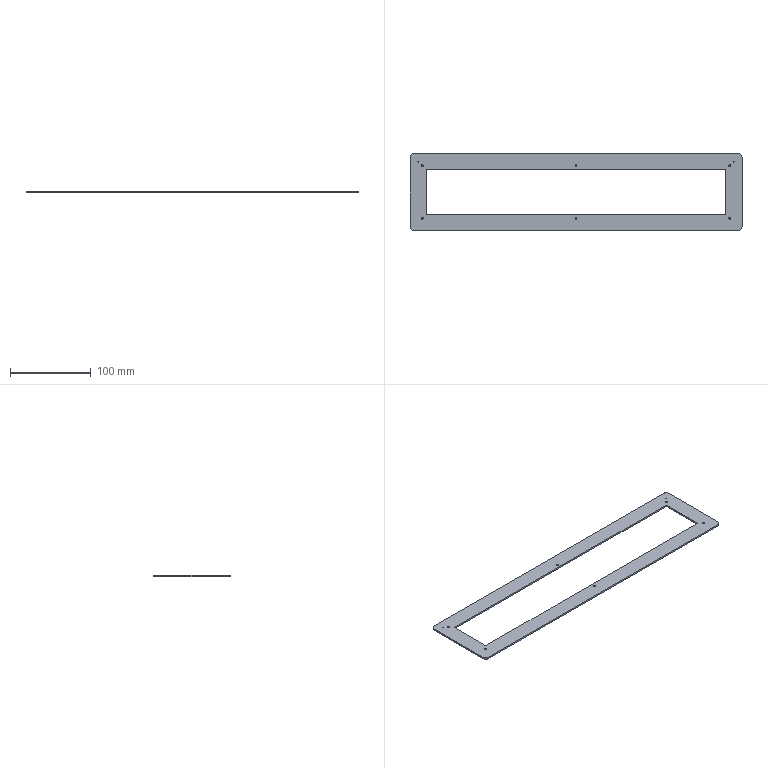Part | NX | features solid 2 | 1 solid | 30 faces | box 410 x 95 x 2 mm | volume 37097 mm3 | cylinder 20 | plane 10 | commonest cylinder face diameters 2.459 x12 1 x4 10 x4
STEP:
#1=CARTESIAN_POINT('',(-455.,-1595.5,1023.));
#2=VERTEX_POINT('',#1);
#3=CARTESIAN_POINT('',(-455.,-1595.5,1021.));
#4=VERTEX_POINT('',#3);
#5=CARTESIAN_POINT('',(-455.,-1595.5,602.133));
#6=DIRECTION('',(0.,0.,1.));
#7=VECTOR('',#6,1000.);
#8=LINE('',#5,#7);
#9=EDGE_CURVE('',#2,#4,#8,.F.);
#10=ORIENTED_EDGE('',*,*,#9,.T.);
#11=CARTESIAN_POINT('',(-455.,-1594.5,1021.));
#12=VERTEX_POINT('',#11);
#13=CARTESIAN_POINT('',(-455.,-1595.,1021.));
#14=DIRECTION('',(0.,0.,-1.));
#15=DIRECTION('',(0.,-1.,0.));
#16=AXIS2_PLACEMENT_3D('',#13,#14,#15);
#17=CIRCLE('',#16,0.5);
#18=EDGE_CURVE('',#4,#12,#17,.T.);
#19=ORIENTED_EDGE('',*,*,#18,.T.);
#20=CARTESIAN_POINT('',(-455.,-1594.5,1023.));
#21=VERTEX_POINT('',#20);
#22=CARTESIAN_POINT('',(-455.,-1594.5,602.133));
#23=DIRECTION('',(0.,0.,1.));
#24=VECTOR('',#23,1000.);
#25=LINE('',#22,#24);
#26=EDGE_CURVE('',#12,#21,#25,.T.);
#27=ORIENTED_EDGE('',*,*,#26,.T.);
#28=CARTESIAN_POINT('',(-455.,-1595.,1023.));
#29=DIRECTION('',(0.,0.,1.));
#30=DIRECTION('',(-1.,0.,0.));
#31=AXIS2_PLACEMENT_3D('',#28,#29,#30);
#32=CIRCLE('',#31,0.5);
#33=EDGE_CURVE('',#21,#2,#32,.T.);
#34=ORIENTED_EDGE('',*,*,#33,.T.);
#35=EDGE_LOOP('',(#10,#19,#27,#34));
#36=FACE_BOUND('',#35,.T.);
#37=CARTESIAN_POINT('',(-455.,-1595.,602.133));
#38=DIRECTION('',(0.,0.,1.));
#39=DIRECTION('',(0.,1.,0.));
#40=AXIS2_PLACEMENT_3D('',#37,#38,#39);
#41=CYLINDRICAL_SURFACE('',#40,0.5);
#42=ADVANCED_FACE('',(#36),#41,.F.);
#43=CARTESIAN_POINT('',(-845.,-1595.5,1023.));
#44=VERTEX_POINT('',#43);
#45=CARTESIAN_POINT('',(-845.,-1595.5,1021.));
#46=VERTEX_POINT('',#45);
#47=CARTESIAN_POINT('',(-845.,-1595.5,602.133));
#48=DIRECTION('',(0.,0.,1.));
#49=VECTOR('',#48,1000.);
#50=LINE('',#47,#49);
#51=EDGE_CURVE('',#44,#46,#50,.F.);
#52=ORIENTED_EDGE('',*,*,#51,.T.);
#53=CARTESIAN_POINT('',(-845.,-1594.5,1021.));
#54=VERTEX_POINT('',#53);
#55=CARTESIAN_POINT('',(-845.,-1595.,1021.));
#56=DIRECTION('',(0.,0.,-1.));
#57=DIRECTION('',(0.,-1.,0.));
#58=AXIS2_PLACEMENT_3D('',#55,#56,#57);
#59=CIRCLE('',#58,0.5);
#60=EDGE_CURVE('',#46,#54,#59,.T.);
#61=ORIENTED_EDGE('',*,*,#60,.T.);
#62=CARTESIAN_POINT('',(-845.,-1594.5,1023.));
#63=VERTEX_POINT('',#62);
#64=CARTESIAN_POINT('',(-845.,-1594.5,602.133));
#65=DIRECTION('',(0.,0.,1.));
#66=VECTOR('',#65,1000.);
#67=LINE('',#64,#66);
#68=EDGE_CURVE('',#54,#63,#67,.T.);
#69=ORIENTED_EDGE('',*,*,#68,.T.);
#70=CARTESIAN_POINT('',(-845.,-1595.,1023.));
#71=DIRECTION('',(0.,0.,1.));
#72=DIRECTION('',(-1.,0.,0.));
#73=AXIS2_PLACEMENT_3D('',#70,#71,#72);
#74=CIRCLE('',#73,0.5);
#75=EDGE_CURVE('',#63,#44,#74,.T.);
#76=ORIENTED_EDGE('',*,*,#75,.T.);
#77=EDGE_LOOP('',(#52,#61,#69,#76));
#78=FACE_BOUND('',#77,.T.);
#79=CARTESIAN_POINT('',(-845.,-1595.,602.133));
#80=DIRECTION('',(0.,0.,1.));
#81=DIRECTION('',(0.,1.,0.));
#82=AXIS2_PLACEMENT_3D('',#79,#80,#81);
#83=CYLINDRICAL_SURFACE('',#82,0.5);
#84=ADVANCED_FACE('',(#78),#83,.F.);
#85=CARTESIAN_POINT('',(-460.,-1598.771,1023.));
#86=VERTEX_POINT('',#85);
#87=CARTESIAN_POINT('',(-460.,-1598.771,1021.));
#88=VERTEX_POINT('',#87);
#89=CARTESIAN_POINT('',(-460.,-1598.771,1441.867));
#90=DIRECTION('',(0.,0.,-1.));
#91=VECTOR('',#90,1000.);
#92=LINE('',#89,#91);
#93=EDGE_CURVE('',#86,#88,#92,.T.);
#94=ORIENTED_EDGE('',*,*,#93,.F.);
#95=CARTESIAN_POINT('',(-460.,-1601.229,1023.));
#96=VERTEX_POINT('',#95);
#97=CARTESIAN_POINT('',(-460.,-1600.,1023.));
#98=DIRECTION('',(0.,0.,-1.));
#99=DIRECTION('',(0.,-1.,0.));
#100=AXIS2_PLACEMENT_3D('',#97,#98,#99);
#101=CIRCLE('',#100,1.23);
#102=EDGE_CURVE('',#96,#86,#101,.T.);
#103=ORIENTED_EDGE('',*,*,#102,.F.);
#104=CARTESIAN_POINT('',(-460.,-1601.229,1021.));
#105=VERTEX_POINT('',#104);
#106=CARTESIAN_POINT('',(-460.,-1601.229,1441.867));
#107=DIRECTION('',(0.,0.,-1.));
#108=VECTOR('',#107,1000.);
#109=LINE('',#106,#108);
#110=EDGE_CURVE('',#105,#96,#109,.F.);
#111=ORIENTED_EDGE('',*,*,#110,.F.);
#112=CARTESIAN_POINT('',(-460.,-1600.,1021.));
#113=DIRECTION('',(0.,0.,-1.));
#114=DIRECTION('',(-1.,0.,0.));
#115=AXIS2_PLACEMENT_3D('',#112,#113,#114);
#116=CIRCLE('',#115,1.23);
#117=EDGE_CURVE('',#105,#88,#116,.T.);
#118=ORIENTED_EDGE('',*,*,#117,.T.);
#119=EDGE_LOOP('',(#94,#103,#111,#118));
#120=FACE_BOUND('',#119,.T.);
#121=CARTESIAN_POINT('',(-460.,-1600.,1441.867));
#122=DIRECTION('',(0.,0.,-1.));
#123=DIRECTION('',(0.,-1.,0.));
#124=AXIS2_PLACEMENT_3D('',#121,#122,#123);
#125=CYLINDRICAL_SURFACE('',#124,1.23);
#126=ADVANCED_FACE('',(#120),#125,.F.);
#127=CARTESIAN_POINT('',(-460.,-1663.771,1023.));
#128=VERTEX_POINT('',#127);
#129=CARTESIAN_POINT('',(-460.,-1663.771,1021.));
#130=VERTEX_POINT('',#129);
#131=CARTESIAN_POINT('',(-460.,-1663.771,1441.867));
#132=DIRECTION('',(0.,0.,-1.));
#133=VECTOR('',#132,1000.);
#134=LINE('',#131,#133);
#135=EDGE_CURVE('',#128,#130,#134,.T.);
#136=ORIENTED_EDGE('',*,*,#135,.F.);
#137=CARTESIAN_POINT('',(-460.,-1666.229,1023.));
#138=VERTEX_POINT('',#137);
#139=CARTESIAN_POINT('',(-460.,-1665.,1023.));
#140=DIRECTION('',(0.,0.,-1.));
#141=DIRECTION('',(0.,-1.,0.));
#142=AXIS2_PLACEMENT_3D('',#139,#140,#141);
#143=CIRCLE('',#142,1.23);
#144=EDGE_CURVE('',#138,#128,#143,.T.);
#145=ORIENTED_EDGE('',*,*,#144,.F.);
#146=CARTESIAN_POINT('',(-460.,-1666.229,1021.));
#147=VERTEX_POINT('',#146);
#148=CARTESIAN_POINT('',(-460.,-1666.229,1441.867));
#149=DIRECTION('',(0.,0.,-1.));
#150=VECTOR('',#149,1000.);
#151=LINE('',#148,#150);
#152=EDGE_CURVE('',#147,#138,#151,.F.);
#153=ORIENTED_EDGE('',*,*,#152,.F.);
#154=CARTESIAN_POINT('',(-460.,-1665.,1021.));
#155=DIRECTION('',(0.,0.,-1.));
#156=DIRECTION('',(-1.,0.,0.));
#157=AXIS2_PLACEMENT_3D('',#154,#155,#156);
#158=CIRCLE('',#157,1.23);
#159=EDGE_CURVE('',#147,#130,#158,.T.);
#160=ORIENTED_EDGE('',*,*,#159,.T.);
#161=EDGE_LOOP('',(#136,#145,#153,#160));
#162=FACE_BOUND('',#161,.T.);
#163=CARTESIAN_POINT('',(-460.,-1665.,1441.867));
#164=DIRECTION('',(0.,0.,-1.));
#165=DIRECTION('',(0.,-1.,0.));
#166=AXIS2_PLACEMENT_3D('',#163,#164,#165);
#167=CYLINDRICAL_SURFACE('',#166,1.23);
#168=ADVANCED_FACE('',(#162),#167,.F.);
#169=CARTESIAN_POINT('',(-650.,-1663.771,1021.));
#170=VERTEX_POINT('',#169);
#171=CARTESIAN_POINT('',(-650.,-1663.771,1023.));
#172=VERTEX_POINT('',#171);
#173=CARTESIAN_POINT('',(-650.,-1663.771,1441.867));
#174=DIRECTION('',(0.,0.,-1.));
#175=VECTOR('',#174,1000.);
#176=LINE('',#173,#175);
#177=EDGE_CURVE('',#170,#172,#176,.F.);
#178=ORIENTED_EDGE('',*,*,#177,.T.);
#179=CARTESIAN_POINT('',(-650.,-1666.229,1023.));
#180=VERTEX_POINT('',#179);
#181=CARTESIAN_POINT('',(-650.,-1665.,1023.));
#182=DIRECTION('',(0.,0.,-1.));
#183=DIRECTION('',(0.,-1.,0.));
#184=AXIS2_PLACEMENT_3D('',#181,#182,#183);
#185=CIRCLE('',#184,1.23);
#186=EDGE_CURVE('',#180,#172,#185,.T.);
#187=ORIENTED_EDGE('',*,*,#186,.F.);
#188=CARTESIAN_POINT('',(-650.,-1666.229,1021.));
#189=VERTEX_POINT('',#188);
#190=CARTESIAN_POINT('',(-650.,-1666.229,1441.867));
#191=DIRECTION('',(0.,0.,-1.));
#192=VECTOR('',#191,1000.);
#193=LINE('',#190,#192);
#194=EDGE_CURVE('',#180,#189,#193,.T.);
#195=ORIENTED_EDGE('',*,*,#194,.T.);
#196=CARTESIAN_POINT('',(-650.,-1665.,1021.));
#197=DIRECTION('',(0.,0.,-1.));
#198=DIRECTION('',(-1.,0.,0.));
#199=AXIS2_PLACEMENT_3D('',#196,#197,#198);
#200=CIRCLE('',#199,1.23);
#201=EDGE_CURVE('',#189,#170,#200,.T.);
#202=ORIENTED_EDGE('',*,*,#201,.T.);
#203=EDGE_LOOP('',(#178,#187,#195,#202));
#204=FACE_BOUND('',#203,.T.);
#205=CARTESIAN_POINT('',(-650.,-1665.,1441.867));
#206=DIRECTION('',(0.,0.,-1.));
#207=DIRECTION('',(0.,-1.,0.));
#208=AXIS2_PLACEMENT_3D('',#205,#206,#207);
#209=CYLINDRICAL_SURFACE('',#208,1.23);
#210=ADVANCED_FACE('',(#204),#209,.F.);
#211=CARTESIAN_POINT('',(-840.,-1663.771,1021.));
#212=VERTEX_POINT('',#211);
#213=CARTESIAN_POINT('',(-840.,-1663.771,1023.));
#214=VERTEX_POINT('',#213);
#215=CARTESIAN_POINT('',(-840.,-1663.771,1441.867));
#216=DIRECTION('',(0.,0.,-1.));
#217=VECTOR('',#216,1000.);
#218=LINE('',#215,#217);
#219=EDGE_CURVE('',#212,#214,#218,.F.);
#220=ORIENTED_EDGE('',*,*,#219,.T.);
#221=CARTESIAN_POINT('',(-840.,-1666.229,1023.));
#222=VERTEX_POINT('',#221);
#223=CARTESIAN_POINT('',(-840.,-1665.,1023.));
#224=DIRECTION('',(0.,0.,-1.));
#225=DIRECTION('',(0.,-1.,0.));
#226=AXIS2_PLACEMENT_3D('',#223,#224,#225);
#227=CIRCLE('',#226,1.23);
#228=EDGE_CURVE('',#222,#214,#227,.T.);
#229=ORIENTED_EDGE('',*,*,#228,.F.);
#230=CARTESIAN_POINT('',(-840.,-1666.229,1021.));
#231=VERTEX_POINT('',#230);
#232=CARTESIAN_POINT('',(-840.,-1666.229,1441.867));
#233=DIRECTION('',(0.,0.,-1.));
#234=VECTOR('',#233,1000.);
#235=LINE('',#232,#234);
#236=EDGE_CURVE('',#222,#231,#235,.T.);
#237=ORIENTED_EDGE('',*,*,#236,.T.);
#238=CARTESIAN_POINT('',(-840.,-1665.,1021.));
#239=DIRECTION('',(0.,0.,-1.));
#240=DIRECTION('',(-1.,0.,0.));
#241=AXIS2_PLACEMENT_3D('',#238,#239,#240);
#242=CIRCLE('',#241,1.23);
#243=EDGE_CURVE('',#231,#212,#242,.T.);
#244=ORIENTED_EDGE('',*,*,#243,.T.);
#245=EDGE_LOOP('',(#220,#229,#237,#244));
#246=FACE_BOUND('',#245,.T.);
#247=CARTESIAN_POINT('',(-840.,-1665.,1441.867));
#248=DIRECTION('',(0.,0.,-1.));
#249=DIRECTION('',(0.,-1.,0.));
#250=AXIS2_PLACEMENT_3D('',#247,#248,#249);
#251=CYLINDRICAL_SURFACE('',#250,1.23);
#252=ADVANCED_FACE('',(#246),#251,.F.);
#253=CARTESIAN_POINT('',(-840.,-1598.771,1021.));
#254=VERTEX_POINT('',#253);
#255=CARTESIAN_POINT('',(-840.,-1598.771,1023.));
#256=VERTEX_POINT('',#255);
#257=CARTESIAN_POINT('',(-840.,-1598.771,1441.867));
#258=DIRECTION('',(0.,0.,-1.));
#259=VECTOR('',#258,1000.);
#260=LINE('',#257,#259);
#261=EDGE_CURVE('',#254,#256,#260,.F.);
#262=ORIENTED_EDGE('',*,*,#261,.T.);
#263=CARTESIAN_POINT('',(-840.,-1601.229,1023.));
#264=VERTEX_POINT('',#263);
#265=CARTESIAN_POINT('',(-840.,-1600.,1023.));
#266=DIRECTION('',(0.,0.,-1.));
#267=DIRECTION('',(0.,-1.,0.));
#268=AXIS2_PLACEMENT_3D('',#265,#266,#267);
#269=CIRCLE('',#268,1.23);
#270=EDGE_CURVE('',#264,#256,#269,.T.);
#271=ORIENTED_EDGE('',*,*,#270,.F.);
#272=CARTESIAN_POINT('',(-840.,-1601.229,1021.));
#273=VERTEX_POINT('',#272);
#274=CARTESIAN_POINT('',(-840.,-1601.229,1441.867));
#275=DIRECTION('',(0.,0.,-1.));
#276=VECTOR('',#275,1000.);
#277=LINE('',#274,#276);
#278=EDGE_CURVE('',#264,#273,#277,.T.);
#279=ORIENTED_EDGE('',*,*,#278,.T.);
#280=CARTESIAN_POINT('',(-840.,-1600.,1021.));
#281=DIRECTION('',(0.,0.,-1.));
#282=DIRECTION('',(-1.,0.,0.));
#283=AXIS2_PLACEMENT_3D('',#280,#281,#282);
#284=CIRCLE('',#283,1.23);
#285=EDGE_CURVE('',#273,#254,#284,.T.);
#286=ORIENTED_EDGE('',*,*,#285,.T.);
#287=EDGE_LOOP('',(#262,#271,#279,#286));
#288=FACE_BOUND('',#287,.T.);
#289=CARTESIAN_POINT('',(-840.,-1600.,1441.867));
#290=DIRECTION('',(0.,0.,-1.));
#291=DIRECTION('',(0.,-1.,0.));
#292=AXIS2_PLACEMENT_3D('',#289,#290,#291);
#293=CYLINDRICAL_SURFACE('',#292,1.23);
#294=ADVANCED_FACE('',(#288),#293,.F.);
#295=CARTESIAN_POINT('',(-650.,-1598.771,1021.));
#296=VERTEX_POINT('',#295);
#297=CARTESIAN_POINT('',(-650.,-1598.771,1023.));
#298=VERTEX_POINT('',#297);
#299=CARTESIAN_POINT('',(-650.,-1598.771,1441.867));
#300=DIRECTION('',(0.,0.,-1.));
#301=VECTOR('',#300,1000.);
#302=LINE('',#299,#301);
#303=EDGE_CURVE('',#296,#298,#302,.F.);
#304=ORIENTED_EDGE('',*,*,#303,.T.);
#305=CARTESIAN_POINT('',(-650.,-1601.229,1023.));
#306=VERTEX_POINT('',#305);
#307=CARTESIAN_POINT('',(-650.,-1600.,1023.));
#308=DIRECTION('',(0.,0.,-1.));
#309=DIRECTION('',(0.,-1.,0.));
#310=AXIS2_PLACEMENT_3D('',#307,#308,#309);
#311=CIRCLE('',#310,1.23);
#312=EDGE_CURVE('',#306,#298,#311,.T.);
#313=ORIENTED_EDGE('',*,*,#312,.F.);
#314=CARTESIAN_POINT('',(-650.,-1601.229,1021.));
#315=VERTEX_POINT('',#314);
#316=CARTESIAN_POINT('',(-650.,-1601.229,1441.867));
#317=DIRECTION('',(0.,0.,-1.));
#318=VECTOR('',#317,1000.);
#319=LINE('',#316,#318);
#320=EDGE_CURVE('',#306,#315,#319,.T.);
#321=ORIENTED_EDGE('',*,*,#320,.T.);
#322=CARTESIAN_POINT('',(-650.,-1600.,1021.));
#323=DIRECTION('',(0.,0.,-1.));
#324=DIRECTION('',(-1.,0.,0.));
#325=AXIS2_PLACEMENT_3D('',#322,#323,#324);
#326=CIRCLE('',#325,1.23);
#327=EDGE_CURVE('',#315,#296,#326,.T.);
#328=ORIENTED_EDGE('',*,*,#327,.T.);
#329=EDGE_LOOP('',(#304,#313,#321,#328));
#330=FACE_BOUND('',#329,.T.);
#331=CARTESIAN_POINT('',(-650.,-1600.,1441.867));
#332=DIRECTION('',(0.,0.,-1.));
#333=DIRECTION('',(0.,-1.,0.));
#334=AXIS2_PLACEMENT_3D('',#331,#332,#333);
#335=CYLINDRICAL_SURFACE('',#334,1.23);
#336=ADVANCED_FACE('',(#330),#335,.F.);
#337=CARTESIAN_POINT('',(-850.,-1585.,1023.));
#338=VERTEX_POINT('',#337);
#339=CARTESIAN_POINT('',(-855.,-1590.,1023.));
#340=VERTEX_POINT('',#339);
#341=CARTESIAN_POINT('',(-850.,-1590.,1023.));
#342=DIRECTION('',(0.,0.,1.));
#343=DIRECTION('',(0.,-1.,0.));
#344=AXIS2_PLACEMENT_3D('',#341,#342,#343);
#345=CIRCLE('',#344,5.);
#346=EDGE_CURVE('',#338,#340,#345,.T.);
#347=ORIENTED_EDGE('',*,*,#346,.F.);
#348=CARTESIAN_POINT('',(-850.,-1585.,1021.));
#349=VERTEX_POINT('',#348);
#350=CARTESIAN_POINT('',(-850.,-1585.,1023.));
#351=DIRECTION('',(0.,0.,1.));
#352=VECTOR('',#351,1000.);
#353=LINE('',#350,#352);
#354=EDGE_CURVE('',#349,#338,#353,.T.);
#355=ORIENTED_EDGE('',*,*,#354,.F.);
#356=CARTESIAN_POINT('',(-855.,-1590.,1021.));
#357=VERTEX_POINT('',#356);
#358=CARTESIAN_POINT('',(-850.,-1590.,1021.));
#359=DIRECTION('',(0.,0.,-1.));
#360=DIRECTION('',(0.,-1.,0.));
#361=AXIS2_PLACEMENT_3D('',#358,#359,#360);
#362=CIRCLE('',#361,5.);
#363=EDGE_CURVE('',#357,#349,#362,.T.);
#364=ORIENTED_EDGE('',*,*,#363,.F.);
#365=CARTESIAN_POINT('',(-855.,-1590.,1023.));
#366=DIRECTION('',(0.,0.,-1.));
#367=VECTOR('',#366,1000.);
#368=LINE('',#365,#367);
#369=EDGE_CURVE('',#340,#357,#368,.T.);
#370=ORIENTED_EDGE('',*,*,#369,.F.);
#371=EDGE_LOOP('',(#347,#355,#364,#370));
#372=FACE_BOUND('',#371,.T.);
#373=CARTESIAN_POINT('',(-850.,-1590.,1023.));
#374=DIRECTION('',(0.,0.,-1.));
#375=DIRECTION('',(0.,-1.,0.));
#376=AXIS2_PLACEMENT_3D('',#373,#374,#375);
#377=CYLINDRICAL_SURFACE('',#376,5.);
#378=ADVANCED_FACE('',(#372),#377,.T.);
#379=CARTESIAN_POINT('',(-450.,-1680.,1023.));
#380=VERTEX_POINT('',#379);
#381=CARTESIAN_POINT('',(-445.,-1675.,1023.));
#382=VERTEX_POINT('',#381);
#383=CARTESIAN_POINT('',(-450.,-1675.,1023.));
#384=DIRECTION('',(0.,0.,1.));
#385=DIRECTION('',(0.,-1.,0.));
#386=AXIS2_PLACEMENT_3D('',#383,#384,#385);
#387=CIRCLE('',#386,5.);
#388=EDGE_CURVE('',#380,#382,#387,.T.);
#389=ORIENTED_EDGE('',*,*,#388,.F.);
#390=CARTESIAN_POINT('',(-450.,-1680.,1021.));
#391=VERTEX_POINT('',#390);
#392=CARTESIAN_POINT('',(-450.,-1680.,1023.));
#393=DIRECTION('',(0.,0.,1.));
#394=VECTOR('',#393,1000.);
#395=LINE('',#392,#394);
#396=EDGE_CURVE('',#391,#380,#395,.T.);
#397=ORIENTED_EDGE('',*,*,#396,.F.);
#398=CARTESIAN_POINT('',(-445.,-1675.,1021.));
#399=VERTEX_POINT('',#398);
#400=CARTESIAN_POINT('',(-450.,-1675.,1021.));
#401=DIRECTION('',(0.,0.,-1.));
#402=DIRECTION('',(0.,-1.,0.));
#403=AXIS2_PLACEMENT_3D('',#400,#401,#402);
#404=CIRCLE('',#403,5.);
#405=EDGE_CURVE('',#399,#391,#404,.T.);
#406=ORIENTED_EDGE('',*,*,#405,.F.);
#407=CARTESIAN_POINT('',(-445.,-1675.,1023.));
#408=DIRECTION('',(0.,0.,-1.));
#409=VECTOR('',#408,1000.);
#410=LINE('',#407,#409);
#411=EDGE_CURVE('',#382,#399,#410,.T.);
#412=ORIENTED_EDGE('',*,*,#411,.F.);
#413=EDGE_LOOP('',(#389,#397,#406,#412));
#414=FACE_BOUND('',#413,.T.);
#415=CARTESIAN_POINT('',(-450.,-1675.,1023.));
#416=DIRECTION('',(0.,0.,-1.));
#417=DIRECTION('',(0.,-1.,0.));
#418=AXIS2_PLACEMENT_3D('',#415,#416,#417);
#419=CYLINDRICAL_SURFACE('',#418,5.);
#420=ADVANCED_FACE('',(#414),#419,.T.);
#421=CARTESIAN_POINT('',(-445.,-1590.,1023.));
#422=VERTEX_POINT('',#421);
#423=CARTESIAN_POINT('',(-450.,-1585.,1023.));
#424=VERTEX_POINT('',#423);
#425=CARTESIAN_POINT('',(-450.,-1590.,1023.));
#426=DIRECTION('',(0.,0.,1.));
#427=DIRECTION('',(0.,-1.,0.));
#428=AXIS2_PLACEMENT_3D('',#425,#426,#427);
#429=CIRCLE('',#428,5.);
#430=EDGE_CURVE('',#422,#424,#429,.T.);
#431=ORIENTED_EDGE('',*,*,#430,.F.);
#432=CARTESIAN_POINT('',(-445.,-1590.,1021.));
#433=VERTEX_POINT('',#432);
#434=CARTESIAN_POINT('',(-445.,-1590.,1023.));
#435=DIRECTION('',(0.,0.,1.));
#436=VECTOR('',#435,1000.);
#437=LINE('',#434,#436);
#438=EDGE_CURVE('',#433,#422,#437,.T.);
#439=ORIENTED_EDGE('',*,*,#438,.F.);
#440=CARTESIAN_POINT('',(-450.,-1585.,1021.));
#441=VERTEX_POINT('',#440);
#442=CARTESIAN_POINT('',(-450.,-1590.,1021.));
#443=DIRECTION('',(0.,0.,-1.));
#444=DIRECTION('',(0.,-1.,0.));
#445=AXIS2_PLACEMENT_3D('',#442,#443,#444);
#446=CIRCLE('',#445,5.);
#447=EDGE_CURVE('',#441,#433,#446,.T.);
#448=ORIENTED_EDGE('',*,*,#447,.F.);
#449=CARTESIAN_POINT('',(-450.,-1585.,1023.));
#450=DIRECTION('',(0.,0.,-1.));
#451=VECTOR('',#450,1000.);
#452=LINE('',#449,#451);
#453=EDGE_CURVE('',#424,#441,#452,.T.);
#454=ORIENTED_EDGE('',*,*,#453,.F.);
#455=EDGE_LOOP('',(#431,#439,#448,#454));
#456=FACE_BOUND('',#455,.T.);
#457=CARTESIAN_POINT('',(-450.,-1590.,1023.));
#458=DIRECTION('',(0.,0.,-1.));
#459=DIRECTION('',(0.,-1.,0.));
#460=AXIS2_PLACEMENT_3D('',#457,#458,#459);
#461=CYLINDRICAL_SURFACE('',#460,5.);
#462=ADVANCED_FACE('',(#456),#461,.T.);
#463=CARTESIAN_POINT('',(-855.,-1675.,1023.));
#464=VERTEX_POINT('',#463);
#465=CARTESIAN_POINT('',(-850.,-1680.,1023.));
#466=VERTEX_POINT('',#465);
#467=CARTESIAN_POINT('',(-850.,-1675.,1023.));
#468=DIRECTION('',(0.,0.,1.));
#469=DIRECTION('',(0.,-1.,0.));
#470=AXIS2_PLACEMENT_3D('',#467,#468,#469);
#471=CIRCLE('',#470,5.);
#472=EDGE_CURVE('',#464,#466,#471,.T.);
#473=ORIENTED_EDGE('',*,*,#472,.F.);
#474=CARTESIAN_POINT('',(-855.,-1675.,1021.));
#475=VERTEX_POINT('',#474);
#476=CARTESIAN_POINT('',(-855.,-1675.,1023.));
#477=DIRECTION('',(0.,0.,1.));
#478=VECTOR('',#477,1000.);
#479=LINE('',#476,#478);
#480=EDGE_CURVE('',#475,#464,#479,.T.);
#481=ORIENTED_EDGE('',*,*,#480,.F.);
#482=CARTESIAN_POINT('',(-850.,-1680.,1021.));
#483=VERTEX_POINT('',#482);
#484=CARTESIAN_POINT('',(-850.,-1675.,1021.));
#485=DIRECTION('',(0.,0.,-1.));
#486=DIRECTION('',(0.,-1.,0.));
#487=AXIS2_PLACEMENT_3D('',#484,#485,#486);
#488=CIRCLE('',#487,5.);
#489=EDGE_CURVE('',#483,#475,#488,.T.);
#490=ORIENTED_EDGE('',*,*,#489,.F.);
#491=CARTESIAN_POINT('',(-850.,-1680.,1023.));
#492=DIRECTION('',(0.,0.,-1.));
#493=VECTOR('',#492,1000.);
#494=LINE('',#491,#493);
#495=EDGE_CURVE('',#466,#483,#494,.T.);
#496=ORIENTED_EDGE('',*,*,#495,.F.);
#497=EDGE_LOOP('',(#473,#481,#490,#496));
#498=FACE_BOUND('',#497,.T.);
#499=CARTESIAN_POINT('',(-850.,-1675.,1023.));
#500=DIRECTION('',(0.,0.,-1.));
#501=DIRECTION('',(0.,-1.,0.));
#502=AXIS2_PLACEMENT_3D('',#499,#500,#501);
#503=CYLINDRICAL_SURFACE('',#502,5.);
#504=ADVANCED_FACE('',(#498),#503,.T.);
#505=CARTESIAN_POINT('',(-835.,-1605.,1023.));
#506=VERTEX_POINT('',#505);
#507=CARTESIAN_POINT('',(-835.,-1605.,1021.));
#508=VERTEX_POINT('',#507);
#509=CARTESIAN_POINT('',(-835.,-1605.,1441.867));
#510=DIRECTION('',(0.,0.,-1.));
#511=VECTOR('',#510,1000.);
#512=LINE('',#509,#511);
#513=EDGE_CURVE('',#506,#508,#512,.T.);
#514=ORIENTED_EDGE('',*,*,#513,.T.);
#515=CARTESIAN_POINT('',(-465.,-1605.,1021.));
#516=VERTEX_POINT('',#515);
#517=CARTESIAN_POINT('',(-835.,-1605.,1021.));
#518=DIRECTION('',(1.,0.,0.));
#519=VECTOR('',#518,1000.);
#520=LINE('',#517,#519);
#521=EDGE_CURVE('',#508,#516,#520,.T.);
#522=ORIENTED_EDGE('',*,*,#521,.T.);
#523=CARTESIAN_POINT('',(-465.,-1605.,1023.));
#524=VERTEX_POINT('',#523);
#525=CARTESIAN_POINT('',(-465.,-1605.,1441.867));
#526=DIRECTION('',(0.,0.,-1.));
#527=VECTOR('',#526,1000.);
#528=LINE('',#525,#527);
#529=EDGE_CURVE('',#524,#516,#528,.T.);
#530=ORIENTED_EDGE('',*,*,#529,.F.);
#531=CARTESIAN_POINT('',(-445.,-1605.,1023.));
#532=DIRECTION('',(1.,0.,0.));
#533=VECTOR('',#532,1000.);
#534=LINE('',#531,#533);
#535=EDGE_CURVE('',#506,#524,#534,.T.);
#536=ORIENTED_EDGE('',*,*,#535,.F.);
#537=EDGE_LOOP('',(#514,#522,#530,#536));
#538=FACE_BOUND('',#537,.T.);
#539=CARTESIAN_POINT('',(-835.,-1605.,1441.867));
#540=DIRECTION('',(0.,1.,0.));
#541=DIRECTION('',(0.,0.,-1.));
#542=AXIS2_PLACEMENT_3D('',#539,#540,#541);
#543=PLANE('',#542);
#544=ADVANCED_FACE('',(#538),#543,.F.);
#545=CARTESIAN_POINT('',(-835.,-1660.,1023.));
#546=VERTEX_POINT('',#545);
#547=CARTESIAN_POINT('',(-835.,-1660.,1021.));
#548=VERTEX_POINT('',#547);
#549=CARTESIAN_POINT('',(-835.,-1660.,1441.867));
#550=DIRECTION('',(0.,0.,-1.));
#551=VECTOR('',#550,1000.);
#552=LINE('',#549,#551);
#553=EDGE_CURVE('',#546,#548,#552,.T.);
#554=ORIENTED_EDGE('',*,*,#553,.T.);
#555=CARTESIAN_POINT('',(-835.,-1660.,1021.));
#556=DIRECTION('',(0.,1.,0.));
#557=VECTOR('',#556,1000.);
#558=LINE('',#555,#557);
#559=EDGE_CURVE('',#548,#508,#558,.T.);
#560=ORIENTED_EDGE('',*,*,#559,.T.);
#561=ORIENTED_EDGE('',*,*,#513,.F.);
#562=CARTESIAN_POINT('',(-835.,-1680.,1023.));
#563=DIRECTION('',(0.,1.,0.));
#564=VECTOR('',#563,1000.);
#565=LINE('',#562,#564);
#566=EDGE_CURVE('',#546,#506,#565,.T.);
#567=ORIENTED_EDGE('',*,*,#566,.F.);
#568=EDGE_LOOP('',(#554,#560,#561,#567));
#569=FACE_BOUND('',#568,.T.);
#570=CARTESIAN_POINT('',(-835.,-1660.,1441.867));
#571=DIRECTION('',(-1.,0.,0.));
#572=DIRECTION('',(0.,1.,0.));
#573=AXIS2_PLACEMENT_3D('',#570,#571,#572);
#574=PLANE('',#573);
#575=ADVANCED_FACE('',(#569),#574,.F.);
#576=CARTESIAN_POINT('',(-465.,-1660.,1023.));
#577=VERTEX_POINT('',#576);
#578=CARTESIAN_POINT('',(-465.,-1660.,1021.));
#579=VERTEX_POINT('',#578);
#580=CARTESIAN_POINT('',(-465.,-1660.,1441.867));
#581=DIRECTION('',(0.,0.,-1.));
#582=VECTOR('',#581,1000.);
#583=LINE('',#580,#582);
#584=EDGE_CURVE('',#577,#579,#583,.T.);
#585=ORIENTED_EDGE('',*,*,#584,.T.);
#586=CARTESIAN_POINT('',(-465.,-1660.,1021.));
#587=DIRECTION('',(-1.,0.,0.));
#588=VECTOR('',#587,1000.);
#589=LINE('',#586,#588);
#590=EDGE_CURVE('',#579,#548,#589,.T.);
#591=ORIENTED_EDGE('',*,*,#590,.T.);
#592=ORIENTED_EDGE('',*,*,#553,.F.);
#593=CARTESIAN_POINT('',(-445.,-1660.,1023.));
#594=DIRECTION('',(-1.,0.,0.));
#595=VECTOR('',#594,1000.);
#596=LINE('',#593,#595);
#597=EDGE_CURVE('',#577,#546,#596,.T.);
#598=ORIENTED_EDGE('',*,*,#597,.F.);
#599=EDGE_LOOP('',(#585,#591,#592,#598));
#600=FACE_BOUND('',#599,.T.);
#601=CARTESIAN_POINT('',(-465.,-1660.,1441.867));
#602=DIRECTION('',(0.,-1.,0.));
#603=DIRECTION('',(-1.,0.,0.));
#604=AXIS2_PLACEMENT_3D('',#601,#602,#603);
#605=PLANE('',#604);
#606=ADVANCED_FACE('',(#600),#605,.F.);
#607=ORIENTED_EDGE('',*,*,#529,.T.);
#608=CARTESIAN_POINT('',(-465.,-1605.,1021.));
#609=DIRECTION('',(0.,-1.,0.));
#610=VECTOR('',#609,1000.);
#611=LINE('',#608,#610);
#612=EDGE_CURVE('',#516,#579,#611,.T.);
#613=ORIENTED_EDGE('',*,*,#612,.T.);
#614=ORIENTED_EDGE('',*,*,#584,.F.);
#615=CARTESIAN_POINT('',(-465.,-1680.,1023.));
#616=DIRECTION('',(0.,-1.,0.));
#617=VECTOR('',#616,1000.);
#618=LINE('',#615,#617);
#619=EDGE_CURVE('',#524,#577,#618,.T.);
#620=ORIENTED_EDGE('',*,*,#619,.F.);
#621=EDGE_LOOP('',(#607,#613,#614,#620));
#622=FACE_BOUND('',#621,.T.);
#623=CARTESIAN_POINT('',(-465.,-1605.,1441.867));
#624=DIRECTION('',(1.,0.,0.));
#625=DIRECTION('',(0.,0.,-1.));
#626=AXIS2_PLACEMENT_3D('',#623,#624,#625);
#627=PLANE('',#626);
#628=ADVANCED_FACE('',(#622),#627,.F.);
#629=ORIENTED_EDGE('',*,*,#612,.F.);
#630=ORIENTED_EDGE('',*,*,#521,.F.);
#631=ORIENTED_EDGE('',*,*,#559,.F.);
#632=ORIENTED_EDGE('',*,*,#590,.F.);
#633=EDGE_LOOP('',(#629,#630,#631,#632));
#634=FACE_BOUND('',#633,.T.);
#635=ORIENTED_EDGE('',*,*,#327,.F.);
#636=CARTESIAN_POINT('',(-650.,-1600.,1021.));
#637=DIRECTION('',(0.,0.,-1.));
#638=DIRECTION('',(-1.,0.,0.));
#639=AXIS2_PLACEMENT_3D('',#636,#637,#638);
#640=CIRCLE('',#639,1.23);
#641=EDGE_CURVE('',#296,#315,#640,.T.);
#642=ORIENTED_EDGE('',*,*,#641,.F.);
#643=EDGE_LOOP('',(#635,#642));
#644=FACE_BOUND('',#643,.T.);
#645=ORIENTED_EDGE('',*,*,#285,.F.);
#646=CARTESIAN_POINT('',(-840.,-1600.,1021.));
#647=DIRECTION('',(0.,0.,-1.));
#648=DIRECTION('',(-1.,0.,0.));
#649=AXIS2_PLACEMENT_3D('',#646,#647,#648);
#650=CIRCLE('',#649,1.23);
#651=EDGE_CURVE('',#254,#273,#650,.T.);
#652=ORIENTED_EDGE('',*,*,#651,.F.);
#653=EDGE_LOOP('',(#645,#652));
#654=FACE_BOUND('',#653,.T.);
#655=ORIENTED_EDGE('',*,*,#243,.F.);
#656=CARTESIAN_POINT('',(-840.,-1665.,1021.));
#657=DIRECTION('',(0.,0.,-1.));
#658=DIRECTION('',(-1.,0.,0.));
#659=AXIS2_PLACEMENT_3D('',#656,#657,#658);
#660=CIRCLE('',#659,1.23);
#661=EDGE_CURVE('',#212,#231,#660,.T.);
#662=ORIENTED_EDGE('',*,*,#661,.F.);
#663=EDGE_LOOP('',(#655,#662));
#664=FACE_BOUND('',#663,.T.);
#665=ORIENTED_EDGE('',*,*,#201,.F.);
#666=CARTESIAN_POINT('',(-650.,-1665.,1021.));
#667=DIRECTION('',(0.,0.,-1.));
#668=DIRECTION('',(-1.,0.,0.));
#669=AXIS2_PLACEMENT_3D('',#666,#667,#668);
#670=CIRCLE('',#669,1.23);
#671=EDGE_CURVE('',#170,#189,#670,.T.);
#672=ORIENTED_EDGE('',*,*,#671,.F.);
#673=EDGE_LOOP('',(#665,#672));
#674=FACE_BOUND('',#673,.T.);
#675=ORIENTED_EDGE('',*,*,#159,.F.);
#676=CARTESIAN_POINT('',(-460.,-1665.,1021.));
#677=DIRECTION('',(0.,0.,-1.));
#678=DIRECTION('',(-1.,0.,0.));
#679=AXIS2_PLACEMENT_3D('',#676,#677,#678);
#680=CIRCLE('',#679,1.23);
#681=EDGE_CURVE('',#130,#147,#680,.T.);
#682=ORIENTED_EDGE('',*,*,#681,.F.);
#683=EDGE_LOOP('',(#675,#682));
#684=FACE_BOUND('',#683,.T.);
#685=ORIENTED_EDGE('',*,*,#117,.F.);
#686=CARTESIAN_POINT('',(-460.,-1600.,1021.));
#687=DIRECTION('',(0.,0.,-1.));
#688=DIRECTION('',(-1.,0.,0.));
#689=AXIS2_PLACEMENT_3D('',#686,#687,#688);
#690=CIRCLE('',#689,1.23);
#691=EDGE_CURVE('',#88,#105,#690,.T.);
#692=ORIENTED_EDGE('',*,*,#691,.F.);
#693=EDGE_LOOP('',(#685,#692));
#694=FACE_BOUND('',#693,.T.);
#695=CARTESIAN_POINT('',(-845.,-1595.,1021.));
#696=DIRECTION('',(0.,0.,-1.));
#697=DIRECTION('',(0.,-1.,0.));
#698=AXIS2_PLACEMENT_3D('',#695,#696,#697);
#699=CIRCLE('',#698,0.5);
#700=EDGE_CURVE('',#54,#46,#699,.T.);
#701=ORIENTED_EDGE('',*,*,#700,.F.);
#702=ORIENTED_EDGE('',*,*,#60,.F.);
#703=EDGE_LOOP('',(#701,#702));
#704=FACE_BOUND('',#703,.T.);
#705=CARTESIAN_POINT('',(-455.,-1595.,1021.));
#706=DIRECTION('',(0.,0.,-1.));
#707=DIRECTION('',(0.,-1.,0.));
#708=AXIS2_PLACEMENT_3D('',#705,#706,#707);
#709=CIRCLE('',#708,0.5);
#710=EDGE_CURVE('',#12,#4,#709,.T.);
#711=ORIENTED_EDGE('',*,*,#710,.F.);
#712=ORIENTED_EDGE('',*,*,#18,.F.);
#713=EDGE_LOOP('',(#711,#712));
#714=FACE_BOUND('',#713,.T.);
#715=CARTESIAN_POINT('',(-445.,-1680.,1021.));
#716=DIRECTION('',(-1.,0.,0.));
#717=VECTOR('',#716,1000.);
#718=LINE('',#715,#717);
#719=EDGE_CURVE('',#391,#483,#718,.T.);
#720=ORIENTED_EDGE('',*,*,#719,.T.);
#721=ORIENTED_EDGE('',*,*,#489,.T.);
#722=CARTESIAN_POINT('',(-855.,-1680.,1021.));
#723=DIRECTION('',(0.,1.,0.));
#724=VECTOR('',#723,1000.);
#725=LINE('',#722,#724);
#726=EDGE_CURVE('',#475,#357,#725,.T.);
#727=ORIENTED_EDGE('',*,*,#726,.T.);
#728=ORIENTED_EDGE('',*,*,#363,.T.);
#729=CARTESIAN_POINT('',(-855.,-1585.,1021.));
#730=DIRECTION('',(1.,0.,0.));
#731=VECTOR('',#730,1000.);
#732=LINE('',#729,#731);
#733=EDGE_CURVE('',#349,#441,#732,.T.);
#734=ORIENTED_EDGE('',*,*,#733,.T.);
#735=ORIENTED_EDGE('',*,*,#447,.T.);
#736=CARTESIAN_POINT('',(-445.,-1585.,1021.));
#737=DIRECTION('',(0.,-1.,0.));
#738=VECTOR('',#737,1000.);
#739=LINE('',#736,#738);
#740=EDGE_CURVE('',#433,#399,#739,.T.);
#741=ORIENTED_EDGE('',*,*,#740,.T.);
#742=ORIENTED_EDGE('',*,*,#405,.T.);
#743=EDGE_LOOP('',(#720,#721,#727,#728,#734,#735,#741,#742));
#744=FACE_BOUND('',#743,.T.);
#745=CARTESIAN_POINT('',(-445.,-1680.,1021.));
#746=DIRECTION('',(0.,0.,-1.));
#747=DIRECTION('',(0.,-1.,0.));
#748=AXIS2_PLACEMENT_3D('',#745,#746,#747);
#749=PLANE('',#748);
#750=ADVANCED_FACE('',(#634,#644,#654,#664,#674,#684,#694,#704,#714,#744),#749,.T.);
#751=ORIENTED_EDGE('',*,*,#535,.T.);
#752=ORIENTED_EDGE('',*,*,#619,.T.);
#753=ORIENTED_EDGE('',*,*,#597,.T.);
#754=ORIENTED_EDGE('',*,*,#566,.T.);
#755=EDGE_LOOP('',(#751,#752,#753,#754));
#756=FACE_BOUND('',#755,.T.);
#757=ORIENTED_EDGE('',*,*,#312,.T.);
#758=CARTESIAN_POINT('',(-650.,-1600.,1023.));
#759=DIRECTION('',(0.,0.,-1.));
#760=DIRECTION('',(0.,-1.,0.));
#761=AXIS2_PLACEMENT_3D('',#758,#759,#760);
#762=CIRCLE('',#761,1.23);
#763=EDGE_CURVE('',#298,#306,#762,.T.);
#764=ORIENTED_EDGE('',*,*,#763,.T.);
#765=EDGE_LOOP('',(#757,#764));
#766=FACE_BOUND('',#765,.T.);
#767=ORIENTED_EDGE('',*,*,#270,.T.);
#768=CARTESIAN_POINT('',(-840.,-1600.,1023.));
#769=DIRECTION('',(0.,0.,-1.));
#770=DIRECTION('',(0.,-1.,0.));
#771=AXIS2_PLACEMENT_3D('',#768,#769,#770);
#772=CIRCLE('',#771,1.23);
#773=EDGE_CURVE('',#256,#264,#772,.T.);
#774=ORIENTED_EDGE('',*,*,#773,.T.);
#775=EDGE_LOOP('',(#767,#774));
#776=FACE_BOUND('',#775,.T.);
#777=ORIENTED_EDGE('',*,*,#228,.T.);
#778=CARTESIAN_POINT('',(-840.,-1665.,1023.));
#779=DIRECTION('',(0.,0.,-1.));
#780=DIRECTION('',(0.,-1.,0.));
#781=AXIS2_PLACEMENT_3D('',#778,#779,#780);
#782=CIRCLE('',#781,1.23);
#783=EDGE_CURVE('',#214,#222,#782,.T.);
#784=ORIENTED_EDGE('',*,*,#783,.T.);
#785=EDGE_LOOP('',(#777,#784));
#786=FACE_BOUND('',#785,.T.);
#787=ORIENTED_EDGE('',*,*,#186,.T.);
#788=CARTESIAN_POINT('',(-650.,-1665.,1023.));
#789=DIRECTION('',(0.,0.,-1.));
#790=DIRECTION('',(0.,-1.,0.));
#791=AXIS2_PLACEMENT_3D('',#788,#789,#790);
#792=CIRCLE('',#791,1.23);
#793=EDGE_CURVE('',#172,#180,#792,.T.);
#794=ORIENTED_EDGE('',*,*,#793,.T.);
#795=EDGE_LOOP('',(#787,#794));
#796=FACE_BOUND('',#795,.T.);
#797=ORIENTED_EDGE('',*,*,#144,.T.);
#798=CARTESIAN_POINT('',(-460.,-1665.,1023.));
#799=DIRECTION('',(0.,0.,-1.));
#800=DIRECTION('',(0.,-1.,0.));
#801=AXIS2_PLACEMENT_3D('',#798,#799,#800);
#802=CIRCLE('',#801,1.23);
#803=EDGE_CURVE('',#128,#138,#802,.T.);
#804=ORIENTED_EDGE('',*,*,#803,.T.);
#805=EDGE_LOOP('',(#797,#804));
#806=FACE_BOUND('',#805,.T.);
#807=ORIENTED_EDGE('',*,*,#102,.T.);
#808=CARTESIAN_POINT('',(-460.,-1600.,1023.));
#809=DIRECTION('',(0.,0.,-1.));
#810=DIRECTION('',(0.,-1.,0.));
#811=AXIS2_PLACEMENT_3D('',#808,#809,#810);
#812=CIRCLE('',#811,1.23);
#813=EDGE_CURVE('',#86,#96,#812,.T.);
#814=ORIENTED_EDGE('',*,*,#813,.T.);
#815=EDGE_LOOP('',(#807,#814));
#816=FACE_BOUND('',#815,.T.);
#817=ORIENTED_EDGE('',*,*,#75,.F.);
#818=CARTESIAN_POINT('',(-845.,-1595.,1023.));
#819=DIRECTION('',(0.,0.,1.));
#820=DIRECTION('',(-1.,0.,0.));
#821=AXIS2_PLACEMENT_3D('',#818,#819,#820);
#822=CIRCLE('',#821,0.5);
#823=EDGE_CURVE('',#44,#63,#822,.T.);
#824=ORIENTED_EDGE('',*,*,#823,.F.);
#825=EDGE_LOOP('',(#817,#824));
#826=FACE_BOUND('',#825,.T.);
#827=ORIENTED_EDGE('',*,*,#33,.F.);
#828=CARTESIAN_POINT('',(-455.,-1595.,1023.));
#829=DIRECTION('',(0.,0.,1.));
#830=DIRECTION('',(-1.,0.,0.));
#831=AXIS2_PLACEMENT_3D('',#828,#829,#830);
#832=CIRCLE('',#831,0.5);
#833=EDGE_CURVE('',#2,#21,#832,.T.);
#834=ORIENTED_EDGE('',*,*,#833,.F.);
#835=EDGE_LOOP('',(#827,#834));
#836=FACE_BOUND('',#835,.T.);
#837=CARTESIAN_POINT('',(-855.,-1680.,1023.));
#838=DIRECTION('',(0.,1.,0.));
#839=VECTOR('',#838,1000.);
#840=LINE('',#837,#839);
#841=EDGE_CURVE('',#464,#340,#840,.T.);
#842=ORIENTED_EDGE('',*,*,#841,.F.);
#843=ORIENTED_EDGE('',*,*,#472,.T.);
#844=CARTESIAN_POINT('',(-445.,-1680.,1023.));
#845=DIRECTION('',(-1.,0.,0.));
#846=VECTOR('',#845,1000.);
#847=LINE('',#844,#846);
#848=EDGE_CURVE('',#380,#466,#847,.T.);
#849=ORIENTED_EDGE('',*,*,#848,.F.);
#850=ORIENTED_EDGE('',*,*,#388,.T.);
#851=CARTESIAN_POINT('',(-445.,-1585.,1023.));
#852=DIRECTION('',(0.,-1.,0.));
#853=VECTOR('',#852,1000.);
#854=LINE('',#851,#853);
#855=EDGE_CURVE('',#422,#382,#854,.T.);
#856=ORIENTED_EDGE('',*,*,#855,.F.);
#857=ORIENTED_EDGE('',*,*,#430,.T.);
#858=CARTESIAN_POINT('',(-855.,-1585.,1023.));
#859=DIRECTION('',(1.,0.,0.));
#860=VECTOR('',#859,1000.);
#861=LINE('',#858,#860);
#862=EDGE_CURVE('',#338,#424,#861,.T.);
#863=ORIENTED_EDGE('',*,*,#862,.F.);
#864=ORIENTED_EDGE('',*,*,#346,.T.);
#865=EDGE_LOOP('',(#842,#843,#849,#850,#856,#857,#863,#864));
#866=FACE_BOUND('',#865,.T.);
#867=CARTESIAN_POINT('',(-445.,-1680.,1023.));
#868=DIRECTION('',(0.,0.,-1.));
#869=DIRECTION('',(0.,-1.,0.));
#870=AXIS2_PLACEMENT_3D('',#867,#868,#869);
#871=PLANE('',#870);
#872=ADVANCED_FACE('',(#756,#766,#776,#786,#796,#806,#816,#826,#836,#866),#871,.F.);
#873=ORIENTED_EDGE('',*,*,#862,.T.);
#874=ORIENTED_EDGE('',*,*,#453,.T.);
#875=ORIENTED_EDGE('',*,*,#733,.F.);
#876=ORIENTED_EDGE('',*,*,#354,.T.);
#877=EDGE_LOOP('',(#873,#874,#875,#876));
#878=FACE_BOUND('',#877,.T.);
#879=CARTESIAN_POINT('',(-855.,-1585.,1023.));
#880=DIRECTION('',(0.,1.,0.));
#881=DIRECTION('',(0.,0.,-1.));
#882=AXIS2_PLACEMENT_3D('',#879,#880,#881);
#883=PLANE('',#882);
#884=ADVANCED_FACE('',(#878),#883,.T.);
#885=ORIENTED_EDGE('',*,*,#726,.F.);
#886=ORIENTED_EDGE('',*,*,#480,.T.);
#887=ORIENTED_EDGE('',*,*,#841,.T.);
#888=ORIENTED_EDGE('',*,*,#369,.T.);
#889=EDGE_LOOP('',(#885,#886,#887,#888));
#890=FACE_BOUND('',#889,.T.);
#891=CARTESIAN_POINT('',(-855.,-1680.,1023.));
#892=DIRECTION('',(-1.,0.,0.));
#893=DIRECTION('',(0.,1.,0.));
#894=AXIS2_PLACEMENT_3D('',#891,#892,#893);
#895=PLANE('',#894);
#896=ADVANCED_FACE('',(#890),#895,.T.);
#897=ORIENTED_EDGE('',*,*,#848,.T.);
#898=ORIENTED_EDGE('',*,*,#495,.T.);
#899=ORIENTED_EDGE('',*,*,#719,.F.);
#900=ORIENTED_EDGE('',*,*,#396,.T.);
#901=EDGE_LOOP('',(#897,#898,#899,#900));
#902=FACE_BOUND('',#901,.T.);
#903=CARTESIAN_POINT('',(-445.,-1680.,1023.));
#904=DIRECTION('',(0.,-1.,0.));
#905=DIRECTION('',(-1.,0.,0.));
#906=AXIS2_PLACEMENT_3D('',#903,#904,#905);
#907=PLANE('',#906);
#908=ADVANCED_FACE('',(#902),#907,.T.);
#909=ORIENTED_EDGE('',*,*,#740,.F.);
#910=ORIENTED_EDGE('',*,*,#438,.T.);
#911=ORIENTED_EDGE('',*,*,#855,.T.);
#912=ORIENTED_EDGE('',*,*,#411,.T.);
#913=EDGE_LOOP('',(#909,#910,#911,#912));
#914=FACE_BOUND('',#913,.T.);
#915=CARTESIAN_POINT('',(-445.,-1585.,1023.));
#916=DIRECTION('',(1.,0.,0.));
#917=DIRECTION('',(0.,0.,-1.));
#918=AXIS2_PLACEMENT_3D('',#915,#916,#917);
#919=PLANE('',#918);
#920=ADVANCED_FACE('',(#914),#919,.T.);
#921=ORIENTED_EDGE('',*,*,#763,.F.);
#922=ORIENTED_EDGE('',*,*,#303,.F.);
#923=ORIENTED_EDGE('',*,*,#641,.T.);
#924=ORIENTED_EDGE('',*,*,#320,.F.);
#925=EDGE_LOOP('',(#921,#922,#923,#924));
#926=FACE_BOUND('',#925,.T.);
#927=CARTESIAN_POINT('',(-650.,-1600.,1441.867));
#928=DIRECTION('',(0.,0.,-1.));
#929=DIRECTION('',(0.,-1.,0.));
#930=AXIS2_PLACEMENT_3D('',#927,#928,#929);
#931=CYLINDRICAL_SURFACE('',#930,1.23);
#932=ADVANCED_FACE('',(#926),#931,.F.);
#933=ORIENTED_EDGE('',*,*,#773,.F.);
#934=ORIENTED_EDGE('',*,*,#261,.F.);
#935=ORIENTED_EDGE('',*,*,#651,.T.);
#936=ORIENTED_EDGE('',*,*,#278,.F.);
#937=EDGE_LOOP('',(#933,#934,#935,#936));
#938=FACE_BOUND('',#937,.T.);
#939=CARTESIAN_POINT('',(-840.,-1600.,1441.867));
#940=DIRECTION('',(0.,0.,-1.));
#941=DIRECTION('',(0.,-1.,0.));
#942=AXIS2_PLACEMENT_3D('',#939,#940,#941);
#943=CYLINDRICAL_SURFACE('',#942,1.23);
#944=ADVANCED_FACE('',(#938),#943,.F.);
#945=ORIENTED_EDGE('',*,*,#783,.F.);
#946=ORIENTED_EDGE('',*,*,#219,.F.);
#947=ORIENTED_EDGE('',*,*,#661,.T.);
#948=ORIENTED_EDGE('',*,*,#236,.F.);
#949=EDGE_LOOP('',(#945,#946,#947,#948));
#950=FACE_BOUND('',#949,.T.);
#951=CARTESIAN_POINT('',(-840.,-1665.,1441.867));
#952=DIRECTION('',(0.,0.,-1.));
#953=DIRECTION('',(0.,-1.,0.));
#954=AXIS2_PLACEMENT_3D('',#951,#952,#953);
#955=CYLINDRICAL_SURFACE('',#954,1.23);
#956=ADVANCED_FACE('',(#950),#955,.F.);
#957=ORIENTED_EDGE('',*,*,#793,.F.);
#958=ORIENTED_EDGE('',*,*,#177,.F.);
#959=ORIENTED_EDGE('',*,*,#671,.T.);
#960=ORIENTED_EDGE('',*,*,#194,.F.);
#961=EDGE_LOOP('',(#957,#958,#959,#960));
#962=FACE_BOUND('',#961,.T.);
#963=CARTESIAN_POINT('',(-650.,-1665.,1441.867));
#964=DIRECTION('',(0.,0.,-1.));
#965=DIRECTION('',(0.,-1.,0.));
#966=AXIS2_PLACEMENT_3D('',#963,#964,#965);
#967=CYLINDRICAL_SURFACE('',#966,1.23);
#968=ADVANCED_FACE('',(#962),#967,.F.);
#969=ORIENTED_EDGE('',*,*,#803,.F.);
#970=ORIENTED_EDGE('',*,*,#135,.T.);
#971=ORIENTED_EDGE('',*,*,#681,.T.);
#972=ORIENTED_EDGE('',*,*,#152,.T.);
#973=EDGE_LOOP('',(#969,#970,#971,#972));
#974=FACE_BOUND('',#973,.T.);
#975=CARTESIAN_POINT('',(-460.,-1665.,1441.867));
#976=DIRECTION('',(0.,0.,-1.));
#977=DIRECTION('',(0.,-1.,0.));
#978=AXIS2_PLACEMENT_3D('',#975,#976,#977);
#979=CYLINDRICAL_SURFACE('',#978,1.23);
#980=ADVANCED_FACE('',(#974),#979,.F.);
#981=ORIENTED_EDGE('',*,*,#813,.F.);
#982=ORIENTED_EDGE('',*,*,#93,.T.);
#983=ORIENTED_EDGE('',*,*,#691,.T.);
#984=ORIENTED_EDGE('',*,*,#110,.T.);
#985=EDGE_LOOP('',(#981,#982,#983,#984));
#986=FACE_BOUND('',#985,.T.);
#987=CARTESIAN_POINT('',(-460.,-1600.,1441.867));
#988=DIRECTION('',(0.,0.,-1.));
#989=DIRECTION('',(0.,-1.,0.));
#990=AXIS2_PLACEMENT_3D('',#987,#988,#989);
#991=CYLINDRICAL_SURFACE('',#990,1.23);
#992=ADVANCED_FACE('',(#986),#991,.F.);
#993=ORIENTED_EDGE('',*,*,#700,.T.);
#994=ORIENTED_EDGE('',*,*,#51,.F.);
#995=ORIENTED_EDGE('',*,*,#823,.T.);
#996=ORIENTED_EDGE('',*,*,#68,.F.);
#997=EDGE_LOOP('',(#993,#994,#995,#996));
#998=FACE_BOUND('',#997,.T.);
#999=CARTESIAN_POINT('',(-845.,-1595.,602.133));
#1000=DIRECTION('',(0.,0.,1.));
#1001=DIRECTION('',(0.,1.,0.));
#1002=AXIS2_PLACEMENT_3D('',#999,#1000,#1001);
#1003=CYLINDRICAL_SURFACE('',#1002,0.5);
#1004=ADVANCED_FACE('',(#998),#1003,.F.);
#1005=ORIENTED_EDGE('',*,*,#710,.T.);
#1006=ORIENTED_EDGE('',*,*,#9,.F.);
#1007=ORIENTED_EDGE('',*,*,#833,.T.);
#1008=ORIENTED_EDGE('',*,*,#26,.F.);
#1009=EDGE_LOOP('',(#1005,#1006,#1007,#1008));
#1010=FACE_BOUND('',#1009,.T.);
#1011=CARTESIAN_POINT('',(-455.,-1595.,602.133));
#1012=DIRECTION('',(0.,0.,1.));
#1013=DIRECTION('',(0.,1.,0.));
#1014=AXIS2_PLACEMENT_3D('',#1011,#1012,#1013);
#1015=CYLINDRICAL_SURFACE('',#1014,0.5);
#1016=ADVANCED_FACE('',(#1010),#1015,.F.);
#1017=CLOSED_SHELL('',(#42,#84,#126,#168,#210,#252,#294,#336,#378,#420,#462,#504,#544,#575,#606,#628,#750,#872,#884,#896,#908,#920,#932,#944,#956,#968,#980,#992,#1004,#1016));
#1018=MANIFOLD_SOLID_BREP('',#1017);
#1019=(LENGTH_UNIT()NAMED_UNIT(*)SI_UNIT(.MILLI.,.METRE.));
#1020=UNCERTAINTY_MEASURE_WITH_UNIT(LENGTH_MEASURE(0.00001),#1019,'','');
#1021=(NAMED_UNIT(*)PLANE_ANGLE_UNIT()SI_UNIT($,.RADIAN.));
#1022=(NAMED_UNIT(*)SI_UNIT($,.STERADIAN.)SOLID_ANGLE_UNIT());
#1023=(GEOMETRIC_REPRESENTATION_CONTEXT(3)GLOBAL_UNCERTAINTY_ASSIGNED_CONTEXT((#1020))GLOBAL_UNIT_ASSIGNED_CONTEXT((#1019,#1021,#1022))REPRESENTATION_CONTEXT('',''));
#1024=ADVANCED_BREP_SHAPE_REPRESENTATION('',(#1018),#1023);